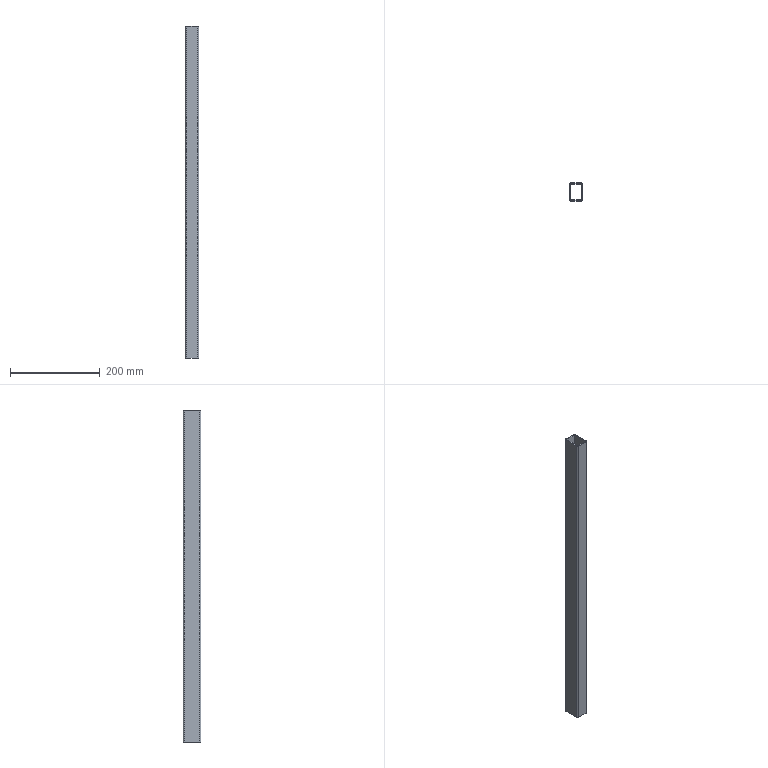Part | SolidWorks | features BaseBody 1 | 1 solid | 18 faces | box 30 x 40 x 740 mm | volume 234942 mm3 | plane 10 | cylinder 8 | commonest cylinder face diameters 1 x4 6 x4
STEP:
#1=CARTESIAN_POINT('',(12.,17.5,-370.));
#2=VERTEX_POINT('',#1);
#3=CARTESIAN_POINT('',(-12.,17.5,-370.));
#4=VERTEX_POINT('',#3);
#5=CARTESIAN_POINT('',(-12.,17.5,-370.));
#6=DIRECTION('',(-1.,0.,0.));
#7=VECTOR('',#6,1000.);
#8=LINE('',#5,#7);
#9=EDGE_CURVE('',#2,#4,#8,.T.);
#10=ORIENTED_EDGE('',*,*,#9,.F.);
#11=CARTESIAN_POINT('',(12.,17.5,370.));
#12=VERTEX_POINT('',#11);
#13=CARTESIAN_POINT('',(12.,17.5,370.));
#14=DIRECTION('',(0.,0.,-1.));
#15=VECTOR('',#14,1000.);
#16=LINE('',#13,#15);
#17=EDGE_CURVE('',#12,#2,#16,.T.);
#18=ORIENTED_EDGE('',*,*,#17,.F.);
#19=CARTESIAN_POINT('',(-12.,17.5,370.));
#20=VERTEX_POINT('',#19);
#21=CARTESIAN_POINT('',(-12.,17.5,370.));
#22=DIRECTION('',(-1.,0.,0.));
#23=VECTOR('',#22,1000.);
#24=LINE('',#21,#23);
#25=EDGE_CURVE('',#12,#20,#24,.T.);
#26=ORIENTED_EDGE('',*,*,#25,.T.);
#27=CARTESIAN_POINT('',(-12.,17.5,370.));
#28=DIRECTION('',(0.,0.,-1.));
#29=VECTOR('',#28,1000.);
#30=LINE('',#27,#29);
#31=EDGE_CURVE('',#20,#4,#30,.T.);
#32=ORIENTED_EDGE('',*,*,#31,.T.);
#33=EDGE_LOOP('',(#10,#18,#26,#32));
#34=FACE_OUTER_BOUND('',#33,.T.);
#35=CARTESIAN_POINT('',(-12.,17.5,370.));
#36=DIRECTION('',(0.,-1.,0.));
#37=DIRECTION('',(0.,0.,-1.));
#38=AXIS2_PLACEMENT_3D('',#35,#36,#37);
#39=PLANE('',#38);
#40=ADVANCED_FACE('',(#34),#39,.T.);
#41=CARTESIAN_POINT('',(12.5,17.,-370.));
#42=VERTEX_POINT('',#41);
#43=CARTESIAN_POINT('',(12.,17.,-370.));
#44=DIRECTION('',(0.,0.,1.));
#45=DIRECTION('',(-1.,0.,0.));
#46=AXIS2_PLACEMENT_3D('',#43,#44,#45);
#47=CIRCLE('',#46,0.5);
#48=EDGE_CURVE('',#42,#2,#47,.T.);
#49=ORIENTED_EDGE('',*,*,#48,.F.);
#50=CARTESIAN_POINT('',(12.5,17.,370.));
#51=VERTEX_POINT('',#50);
#52=CARTESIAN_POINT('',(12.5,17.,370.));
#53=DIRECTION('',(0.,0.,-1.));
#54=VECTOR('',#53,1000.);
#55=LINE('',#52,#54);
#56=EDGE_CURVE('',#51,#42,#55,.T.);
#57=ORIENTED_EDGE('',*,*,#56,.F.);
#58=CARTESIAN_POINT('',(12.,17.,370.));
#59=DIRECTION('',(0.,0.,1.));
#60=DIRECTION('',(-1.,0.,0.));
#61=AXIS2_PLACEMENT_3D('',#58,#59,#60);
#62=CIRCLE('',#61,0.5);
#63=EDGE_CURVE('',#51,#12,#62,.T.);
#64=ORIENTED_EDGE('',*,*,#63,.T.);
#65=ORIENTED_EDGE('',*,*,#17,.T.);
#66=EDGE_LOOP('',(#49,#57,#64,#65));
#67=FACE_OUTER_BOUND('',#66,.T.);
#68=CARTESIAN_POINT('',(12.,17.,370.));
#69=DIRECTION('',(0.,0.,-1.));
#70=DIRECTION('',(-1.,0.,0.));
#71=AXIS2_PLACEMENT_3D('',#68,#69,#70);
#72=CYLINDRICAL_SURFACE('',#71,0.5);
#73=ADVANCED_FACE('',(#67),#72,.F.);
#74=CARTESIAN_POINT('',(12.5,-17.,-370.));
#75=VERTEX_POINT('',#74);
#76=CARTESIAN_POINT('',(12.5,17.,-370.));
#77=DIRECTION('',(0.,1.,0.));
#78=VECTOR('',#77,1000.);
#79=LINE('',#76,#78);
#80=EDGE_CURVE('',#75,#42,#79,.T.);
#81=ORIENTED_EDGE('',*,*,#80,.F.);
#82=CARTESIAN_POINT('',(12.5,-17.,370.));
#83=VERTEX_POINT('',#82);
#84=CARTESIAN_POINT('',(12.5,-17.,370.));
#85=DIRECTION('',(0.,0.,-1.));
#86=VECTOR('',#85,1000.);
#87=LINE('',#84,#86);
#88=EDGE_CURVE('',#83,#75,#87,.T.);
#89=ORIENTED_EDGE('',*,*,#88,.F.);
#90=CARTESIAN_POINT('',(12.5,17.,370.));
#91=DIRECTION('',(0.,1.,0.));
#92=VECTOR('',#91,1000.);
#93=LINE('',#90,#92);
#94=EDGE_CURVE('',#83,#51,#93,.T.);
#95=ORIENTED_EDGE('',*,*,#94,.T.);
#96=ORIENTED_EDGE('',*,*,#56,.T.);
#97=EDGE_LOOP('',(#81,#89,#95,#96));
#98=FACE_OUTER_BOUND('',#97,.T.);
#99=CARTESIAN_POINT('',(12.5,17.,370.));
#100=DIRECTION('',(-1.,0.,0.));
#101=DIRECTION('',(0.,1.,0.));
#102=AXIS2_PLACEMENT_3D('',#99,#100,#101);
#103=PLANE('',#102);
#104=ADVANCED_FACE('',(#98),#103,.T.);
#105=CARTESIAN_POINT('',(12.,-17.5,-370.));
#106=VERTEX_POINT('',#105);
#107=CARTESIAN_POINT('',(12.,-17.,-370.));
#108=DIRECTION('',(0.,0.,1.));
#109=DIRECTION('',(1.,0.,0.));
#110=AXIS2_PLACEMENT_3D('',#107,#108,#109);
#111=CIRCLE('',#110,0.5);
#112=EDGE_CURVE('',#106,#75,#111,.T.);
#113=ORIENTED_EDGE('',*,*,#112,.F.);
#114=CARTESIAN_POINT('',(12.,-17.5,370.));
#115=VERTEX_POINT('',#114);
#116=CARTESIAN_POINT('',(12.,-17.5,370.));
#117=DIRECTION('',(0.,0.,-1.));
#118=VECTOR('',#117,1000.);
#119=LINE('',#116,#118);
#120=EDGE_CURVE('',#115,#106,#119,.T.);
#121=ORIENTED_EDGE('',*,*,#120,.F.);
#122=CARTESIAN_POINT('',(12.,-17.,370.));
#123=DIRECTION('',(0.,0.,1.));
#124=DIRECTION('',(1.,0.,0.));
#125=AXIS2_PLACEMENT_3D('',#122,#123,#124);
#126=CIRCLE('',#125,0.5);
#127=EDGE_CURVE('',#115,#83,#126,.T.);
#128=ORIENTED_EDGE('',*,*,#127,.T.);
#129=ORIENTED_EDGE('',*,*,#88,.T.);
#130=EDGE_LOOP('',(#113,#121,#128,#129));
#131=FACE_OUTER_BOUND('',#130,.T.);
#132=CARTESIAN_POINT('',(12.,-17.,370.));
#133=DIRECTION('',(0.,0.,-1.));
#134=DIRECTION('',(-1.,0.,0.));
#135=AXIS2_PLACEMENT_3D('',#132,#133,#134);
#136=CYLINDRICAL_SURFACE('',#135,0.5);
#137=ADVANCED_FACE('',(#131),#136,.F.);
#138=CARTESIAN_POINT('',(-12.,-17.5,-370.));
#139=VERTEX_POINT('',#138);
#140=CARTESIAN_POINT('',(-12.,-17.5,-370.));
#141=DIRECTION('',(1.,0.,0.));
#142=VECTOR('',#141,1000.);
#143=LINE('',#140,#142);
#144=EDGE_CURVE('',#139,#106,#143,.T.);
#145=ORIENTED_EDGE('',*,*,#144,.F.);
#146=CARTESIAN_POINT('',(-12.,-17.5,370.));
#147=VERTEX_POINT('',#146);
#148=CARTESIAN_POINT('',(-12.,-17.5,370.));
#149=DIRECTION('',(0.,0.,-1.));
#150=VECTOR('',#149,1000.);
#151=LINE('',#148,#150);
#152=EDGE_CURVE('',#147,#139,#151,.T.);
#153=ORIENTED_EDGE('',*,*,#152,.F.);
#154=CARTESIAN_POINT('',(-12.,-17.5,370.));
#155=DIRECTION('',(1.,0.,0.));
#156=VECTOR('',#155,1000.);
#157=LINE('',#154,#156);
#158=EDGE_CURVE('',#147,#115,#157,.T.);
#159=ORIENTED_EDGE('',*,*,#158,.T.);
#160=ORIENTED_EDGE('',*,*,#120,.T.);
#161=EDGE_LOOP('',(#145,#153,#159,#160));
#162=FACE_OUTER_BOUND('',#161,.T.);
#163=CARTESIAN_POINT('',(-12.,-17.5,370.));
#164=DIRECTION('',(0.,1.,0.));
#165=DIRECTION('',(1.,0.,0.));
#166=AXIS2_PLACEMENT_3D('',#163,#164,#165);
#167=PLANE('',#166);
#168=ADVANCED_FACE('',(#162),#167,.T.);
#169=CARTESIAN_POINT('',(-12.5,-17.,-370.));
#170=VERTEX_POINT('',#169);
#171=CARTESIAN_POINT('',(-12.,-17.,-370.));
#172=DIRECTION('',(0.,0.,1.));
#173=DIRECTION('',(1.,0.,0.));
#174=AXIS2_PLACEMENT_3D('',#171,#172,#173);
#175=CIRCLE('',#174,0.5);
#176=EDGE_CURVE('',#170,#139,#175,.T.);
#177=ORIENTED_EDGE('',*,*,#176,.F.);
#178=CARTESIAN_POINT('',(-12.5,-17.,370.));
#179=VERTEX_POINT('',#178);
#180=CARTESIAN_POINT('',(-12.5,-17.,370.));
#181=DIRECTION('',(0.,0.,-1.));
#182=VECTOR('',#181,1000.);
#183=LINE('',#180,#182);
#184=EDGE_CURVE('',#179,#170,#183,.T.);
#185=ORIENTED_EDGE('',*,*,#184,.F.);
#186=CARTESIAN_POINT('',(-12.,-17.,370.));
#187=DIRECTION('',(0.,0.,1.));
#188=DIRECTION('',(1.,0.,0.));
#189=AXIS2_PLACEMENT_3D('',#186,#187,#188);
#190=CIRCLE('',#189,0.5);
#191=EDGE_CURVE('',#179,#147,#190,.T.);
#192=ORIENTED_EDGE('',*,*,#191,.T.);
#193=ORIENTED_EDGE('',*,*,#152,.T.);
#194=EDGE_LOOP('',(#177,#185,#192,#193));
#195=FACE_OUTER_BOUND('',#194,.T.);
#196=CARTESIAN_POINT('',(-12.,-17.,370.));
#197=DIRECTION('',(0.,0.,-1.));
#198=DIRECTION('',(-1.,0.,0.));
#199=AXIS2_PLACEMENT_3D('',#196,#197,#198);
#200=CYLINDRICAL_SURFACE('',#199,0.5);
#201=ADVANCED_FACE('',(#195),#200,.F.);
#202=CARTESIAN_POINT('',(-12.5,17.,-370.));
#203=VERTEX_POINT('',#202);
#204=CARTESIAN_POINT('',(-12.5,17.,-370.));
#205=DIRECTION('',(0.,-1.,0.));
#206=VECTOR('',#205,1000.);
#207=LINE('',#204,#206);
#208=EDGE_CURVE('',#203,#170,#207,.T.);
#209=ORIENTED_EDGE('',*,*,#208,.F.);
#210=CARTESIAN_POINT('',(-12.5,17.,370.));
#211=VERTEX_POINT('',#210);
#212=CARTESIAN_POINT('',(-12.5,17.,370.));
#213=DIRECTION('',(0.,0.,-1.));
#214=VECTOR('',#213,1000.);
#215=LINE('',#212,#214);
#216=EDGE_CURVE('',#211,#203,#215,.T.);
#217=ORIENTED_EDGE('',*,*,#216,.F.);
#218=CARTESIAN_POINT('',(-12.5,17.,370.));
#219=DIRECTION('',(0.,-1.,0.));
#220=VECTOR('',#219,1000.);
#221=LINE('',#218,#220);
#222=EDGE_CURVE('',#211,#179,#221,.T.);
#223=ORIENTED_EDGE('',*,*,#222,.T.);
#224=ORIENTED_EDGE('',*,*,#184,.T.);
#225=EDGE_LOOP('',(#209,#217,#223,#224));
#226=FACE_OUTER_BOUND('',#225,.T.);
#227=CARTESIAN_POINT('',(-12.5,17.,370.));
#228=DIRECTION('',(1.,0.,0.));
#229=DIRECTION('',(0.,1.,0.));
#230=AXIS2_PLACEMENT_3D('',#227,#228,#229);
#231=PLANE('',#230);
#232=ADVANCED_FACE('',(#226),#231,.T.);
#233=CARTESIAN_POINT('',(-12.,17.,-370.));
#234=DIRECTION('',(0.,0.,1.));
#235=DIRECTION('',(1.,0.,0.));
#236=AXIS2_PLACEMENT_3D('',#233,#234,#235);
#237=CIRCLE('',#236,0.5);
#238=EDGE_CURVE('',#4,#203,#237,.T.);
#239=ORIENTED_EDGE('',*,*,#238,.F.);
#240=ORIENTED_EDGE('',*,*,#31,.F.);
#241=CARTESIAN_POINT('',(-12.,17.,370.));
#242=DIRECTION('',(0.,0.,1.));
#243=DIRECTION('',(1.,0.,0.));
#244=AXIS2_PLACEMENT_3D('',#241,#242,#243);
#245=CIRCLE('',#244,0.5);
#246=EDGE_CURVE('',#20,#211,#245,.T.);
#247=ORIENTED_EDGE('',*,*,#246,.T.);
#248=ORIENTED_EDGE('',*,*,#216,.T.);
#249=EDGE_LOOP('',(#239,#240,#247,#248));
#250=FACE_OUTER_BOUND('',#249,.T.);
#251=CARTESIAN_POINT('',(-12.,17.,370.));
#252=DIRECTION('',(0.,0.,-1.));
#253=DIRECTION('',(-1.,0.,0.));
#254=AXIS2_PLACEMENT_3D('',#251,#252,#253);
#255=CYLINDRICAL_SURFACE('',#254,0.5);
#256=ADVANCED_FACE('',(#250),#255,.F.);
#257=CARTESIAN_POINT('',(-15.,17.,-370.));
#258=VERTEX_POINT('',#257);
#259=CARTESIAN_POINT('',(-15.,-17.,-370.));
#260=VERTEX_POINT('',#259);
#261=CARTESIAN_POINT('',(-15.,17.,-370.));
#262=DIRECTION('',(0.,-1.,0.));
#263=VECTOR('',#262,1000.);
#264=LINE('',#261,#263);
#265=EDGE_CURVE('',#258,#260,#264,.T.);
#266=ORIENTED_EDGE('',*,*,#265,.T.);
#267=CARTESIAN_POINT('',(-15.,-17.,370.));
#268=VERTEX_POINT('',#267);
#269=CARTESIAN_POINT('',(-15.,-17.,370.));
#270=DIRECTION('',(0.,0.,-1.));
#271=VECTOR('',#270,1000.);
#272=LINE('',#269,#271);
#273=EDGE_CURVE('',#268,#260,#272,.T.);
#274=ORIENTED_EDGE('',*,*,#273,.F.);
#275=CARTESIAN_POINT('',(-15.,17.,370.));
#276=VERTEX_POINT('',#275);
#277=CARTESIAN_POINT('',(-15.,17.,370.));
#278=DIRECTION('',(0.,-1.,0.));
#279=VECTOR('',#278,1000.);
#280=LINE('',#277,#279);
#281=EDGE_CURVE('',#276,#268,#280,.T.);
#282=ORIENTED_EDGE('',*,*,#281,.F.);
#283=CARTESIAN_POINT('',(-15.,17.,370.));
#284=DIRECTION('',(0.,0.,-1.));
#285=VECTOR('',#284,1000.);
#286=LINE('',#283,#285);
#287=EDGE_CURVE('',#276,#258,#286,.T.);
#288=ORIENTED_EDGE('',*,*,#287,.T.);
#289=EDGE_LOOP('',(#266,#274,#282,#288));
#290=FACE_OUTER_BOUND('',#289,.T.);
#291=CARTESIAN_POINT('',(-15.,17.,370.));
#292=DIRECTION('',(1.,0.,0.));
#293=DIRECTION('',(0.,1.,0.));
#294=AXIS2_PLACEMENT_3D('',#291,#292,#293);
#295=PLANE('',#294);
#296=ADVANCED_FACE('',(#290),#295,.F.);
#297=CARTESIAN_POINT('',(-12.,20.,-370.));
#298=VERTEX_POINT('',#297);
#299=CARTESIAN_POINT('',(-12.,17.,-370.));
#300=DIRECTION('',(0.,0.,1.));
#301=DIRECTION('',(1.,0.,0.));
#302=AXIS2_PLACEMENT_3D('',#299,#300,#301);
#303=CIRCLE('',#302,3.);
#304=EDGE_CURVE('',#298,#258,#303,.T.);
#305=ORIENTED_EDGE('',*,*,#304,.T.);
#306=ORIENTED_EDGE('',*,*,#287,.F.);
#307=CARTESIAN_POINT('',(-12.,20.,370.));
#308=VERTEX_POINT('',#307);
#309=CARTESIAN_POINT('',(-12.,17.,370.));
#310=DIRECTION('',(0.,0.,1.));
#311=DIRECTION('',(1.,0.,0.));
#312=AXIS2_PLACEMENT_3D('',#309,#310,#311);
#313=CIRCLE('',#312,3.);
#314=EDGE_CURVE('',#308,#276,#313,.T.);
#315=ORIENTED_EDGE('',*,*,#314,.F.);
#316=CARTESIAN_POINT('',(-12.,20.,370.));
#317=DIRECTION('',(0.,0.,-1.));
#318=VECTOR('',#317,1000.);
#319=LINE('',#316,#318);
#320=EDGE_CURVE('',#308,#298,#319,.T.);
#321=ORIENTED_EDGE('',*,*,#320,.T.);
#322=EDGE_LOOP('',(#305,#306,#315,#321));
#323=FACE_OUTER_BOUND('',#322,.T.);
#324=CARTESIAN_POINT('',(-12.,17.,370.));
#325=DIRECTION('',(0.,0.,-1.));
#326=DIRECTION('',(-1.,0.,0.));
#327=AXIS2_PLACEMENT_3D('',#324,#325,#326);
#328=CYLINDRICAL_SURFACE('',#327,3.);
#329=ADVANCED_FACE('',(#323),#328,.T.);
#330=CARTESIAN_POINT('',(12.,20.,-370.));
#331=VERTEX_POINT('',#330);
#332=CARTESIAN_POINT('',(-12.,20.,-370.));
#333=DIRECTION('',(-1.,0.,0.));
#334=VECTOR('',#333,1000.);
#335=LINE('',#332,#334);
#336=EDGE_CURVE('',#331,#298,#335,.T.);
#337=ORIENTED_EDGE('',*,*,#336,.T.);
#338=ORIENTED_EDGE('',*,*,#320,.F.);
#339=CARTESIAN_POINT('',(12.,20.,370.));
#340=VERTEX_POINT('',#339);
#341=CARTESIAN_POINT('',(-12.,20.,370.));
#342=DIRECTION('',(-1.,0.,0.));
#343=VECTOR('',#342,1000.);
#344=LINE('',#341,#343);
#345=EDGE_CURVE('',#340,#308,#344,.T.);
#346=ORIENTED_EDGE('',*,*,#345,.F.);
#347=CARTESIAN_POINT('',(12.,20.,370.));
#348=DIRECTION('',(0.,0.,-1.));
#349=VECTOR('',#348,1000.);
#350=LINE('',#347,#349);
#351=EDGE_CURVE('',#340,#331,#350,.T.);
#352=ORIENTED_EDGE('',*,*,#351,.T.);
#353=EDGE_LOOP('',(#337,#338,#346,#352));
#354=FACE_OUTER_BOUND('',#353,.T.);
#355=CARTESIAN_POINT('',(-12.,20.,370.));
#356=DIRECTION('',(0.,-1.,0.));
#357=DIRECTION('',(0.,0.,-1.));
#358=AXIS2_PLACEMENT_3D('',#355,#356,#357);
#359=PLANE('',#358);
#360=ADVANCED_FACE('',(#354),#359,.F.);
#361=CARTESIAN_POINT('',(15.,17.,-370.));
#362=VERTEX_POINT('',#361);
#363=CARTESIAN_POINT('',(12.,17.,-370.));
#364=DIRECTION('',(0.,0.,1.));
#365=DIRECTION('',(-1.,0.,0.));
#366=AXIS2_PLACEMENT_3D('',#363,#364,#365);
#367=CIRCLE('',#366,3.);
#368=EDGE_CURVE('',#362,#331,#367,.T.);
#369=ORIENTED_EDGE('',*,*,#368,.T.);
#370=ORIENTED_EDGE('',*,*,#351,.F.);
#371=CARTESIAN_POINT('',(15.,17.,370.));
#372=VERTEX_POINT('',#371);
#373=CARTESIAN_POINT('',(12.,17.,370.));
#374=DIRECTION('',(0.,0.,1.));
#375=DIRECTION('',(-1.,0.,0.));
#376=AXIS2_PLACEMENT_3D('',#373,#374,#375);
#377=CIRCLE('',#376,3.);
#378=EDGE_CURVE('',#372,#340,#377,.T.);
#379=ORIENTED_EDGE('',*,*,#378,.F.);
#380=CARTESIAN_POINT('',(15.,17.,370.));
#381=DIRECTION('',(0.,0.,-1.));
#382=VECTOR('',#381,1000.);
#383=LINE('',#380,#382);
#384=EDGE_CURVE('',#372,#362,#383,.T.);
#385=ORIENTED_EDGE('',*,*,#384,.T.);
#386=EDGE_LOOP('',(#369,#370,#379,#385));
#387=FACE_OUTER_BOUND('',#386,.T.);
#388=CARTESIAN_POINT('',(12.,17.,370.));
#389=DIRECTION('',(0.,0.,-1.));
#390=DIRECTION('',(-1.,0.,0.));
#391=AXIS2_PLACEMENT_3D('',#388,#389,#390);
#392=CYLINDRICAL_SURFACE('',#391,3.);
#393=ADVANCED_FACE('',(#387),#392,.T.);
#394=CARTESIAN_POINT('',(15.,-17.,-370.));
#395=VERTEX_POINT('',#394);
#396=CARTESIAN_POINT('',(15.,17.,-370.));
#397=DIRECTION('',(0.,1.,0.));
#398=VECTOR('',#397,1000.);
#399=LINE('',#396,#398);
#400=EDGE_CURVE('',#395,#362,#399,.T.);
#401=ORIENTED_EDGE('',*,*,#400,.T.);
#402=ORIENTED_EDGE('',*,*,#384,.F.);
#403=CARTESIAN_POINT('',(15.,-17.,370.));
#404=VERTEX_POINT('',#403);
#405=CARTESIAN_POINT('',(15.,17.,370.));
#406=DIRECTION('',(0.,1.,0.));
#407=VECTOR('',#406,1000.);
#408=LINE('',#405,#407);
#409=EDGE_CURVE('',#404,#372,#408,.T.);
#410=ORIENTED_EDGE('',*,*,#409,.F.);
#411=CARTESIAN_POINT('',(15.,-17.,370.));
#412=DIRECTION('',(0.,0.,-1.));
#413=VECTOR('',#412,1000.);
#414=LINE('',#411,#413);
#415=EDGE_CURVE('',#404,#395,#414,.T.);
#416=ORIENTED_EDGE('',*,*,#415,.T.);
#417=EDGE_LOOP('',(#401,#402,#410,#416));
#418=FACE_OUTER_BOUND('',#417,.T.);
#419=CARTESIAN_POINT('',(15.,17.,370.));
#420=DIRECTION('',(-1.,0.,0.));
#421=DIRECTION('',(0.,1.,0.));
#422=AXIS2_PLACEMENT_3D('',#419,#420,#421);
#423=PLANE('',#422);
#424=ADVANCED_FACE('',(#418),#423,.F.);
#425=CARTESIAN_POINT('',(12.,-20.,-370.));
#426=VERTEX_POINT('',#425);
#427=CARTESIAN_POINT('',(12.,-17.,-370.));
#428=DIRECTION('',(0.,0.,1.));
#429=DIRECTION('',(1.,0.,0.));
#430=AXIS2_PLACEMENT_3D('',#427,#428,#429);
#431=CIRCLE('',#430,3.);
#432=EDGE_CURVE('',#426,#395,#431,.T.);
#433=ORIENTED_EDGE('',*,*,#432,.T.);
#434=ORIENTED_EDGE('',*,*,#415,.F.);
#435=CARTESIAN_POINT('',(12.,-20.,370.));
#436=VERTEX_POINT('',#435);
#437=CARTESIAN_POINT('',(12.,-17.,370.));
#438=DIRECTION('',(0.,0.,1.));
#439=DIRECTION('',(1.,0.,0.));
#440=AXIS2_PLACEMENT_3D('',#437,#438,#439);
#441=CIRCLE('',#440,3.);
#442=EDGE_CURVE('',#436,#404,#441,.T.);
#443=ORIENTED_EDGE('',*,*,#442,.F.);
#444=CARTESIAN_POINT('',(12.,-20.,370.));
#445=DIRECTION('',(0.,0.,-1.));
#446=VECTOR('',#445,1000.);
#447=LINE('',#444,#446);
#448=EDGE_CURVE('',#436,#426,#447,.T.);
#449=ORIENTED_EDGE('',*,*,#448,.T.);
#450=EDGE_LOOP('',(#433,#434,#443,#449));
#451=FACE_OUTER_BOUND('',#450,.T.);
#452=CARTESIAN_POINT('',(12.,-17.,370.));
#453=DIRECTION('',(0.,0.,-1.));
#454=DIRECTION('',(-1.,0.,0.));
#455=AXIS2_PLACEMENT_3D('',#452,#453,#454);
#456=CYLINDRICAL_SURFACE('',#455,3.);
#457=ADVANCED_FACE('',(#451),#456,.T.);
#458=CARTESIAN_POINT('',(-12.,-20.,-370.));
#459=VERTEX_POINT('',#458);
#460=CARTESIAN_POINT('',(-12.,-20.,-370.));
#461=DIRECTION('',(1.,0.,0.));
#462=VECTOR('',#461,1000.);
#463=LINE('',#460,#462);
#464=EDGE_CURVE('',#459,#426,#463,.T.);
#465=ORIENTED_EDGE('',*,*,#464,.T.);
#466=ORIENTED_EDGE('',*,*,#448,.F.);
#467=CARTESIAN_POINT('',(-12.,-20.,370.));
#468=VERTEX_POINT('',#467);
#469=CARTESIAN_POINT('',(-12.,-20.,370.));
#470=DIRECTION('',(1.,0.,0.));
#471=VECTOR('',#470,1000.);
#472=LINE('',#469,#471);
#473=EDGE_CURVE('',#468,#436,#472,.T.);
#474=ORIENTED_EDGE('',*,*,#473,.F.);
#475=CARTESIAN_POINT('',(-12.,-20.,370.));
#476=DIRECTION('',(0.,0.,-1.));
#477=VECTOR('',#476,1000.);
#478=LINE('',#475,#477);
#479=EDGE_CURVE('',#468,#459,#478,.T.);
#480=ORIENTED_EDGE('',*,*,#479,.T.);
#481=EDGE_LOOP('',(#465,#466,#474,#480));
#482=FACE_OUTER_BOUND('',#481,.T.);
#483=CARTESIAN_POINT('',(-12.,-20.,370.));
#484=DIRECTION('',(0.,1.,0.));
#485=DIRECTION('',(1.,0.,0.));
#486=AXIS2_PLACEMENT_3D('',#483,#484,#485);
#487=PLANE('',#486);
#488=ADVANCED_FACE('',(#482),#487,.F.);
#489=CARTESIAN_POINT('',(-12.,-17.,-370.));
#490=DIRECTION('',(0.,0.,1.));
#491=DIRECTION('',(1.,0.,0.));
#492=AXIS2_PLACEMENT_3D('',#489,#490,#491);
#493=CIRCLE('',#492,3.);
#494=EDGE_CURVE('',#260,#459,#493,.T.);
#495=ORIENTED_EDGE('',*,*,#494,.T.);
#496=ORIENTED_EDGE('',*,*,#479,.F.);
#497=CARTESIAN_POINT('',(-12.,-17.,370.));
#498=DIRECTION('',(0.,0.,1.));
#499=DIRECTION('',(1.,0.,0.));
#500=AXIS2_PLACEMENT_3D('',#497,#498,#499);
#501=CIRCLE('',#500,3.);
#502=EDGE_CURVE('',#268,#468,#501,.T.);
#503=ORIENTED_EDGE('',*,*,#502,.F.);
#504=ORIENTED_EDGE('',*,*,#273,.T.);
#505=EDGE_LOOP('',(#495,#496,#503,#504));
#506=FACE_OUTER_BOUND('',#505,.T.);
#507=CARTESIAN_POINT('',(-12.,-17.,370.));
#508=DIRECTION('',(0.,0.,-1.));
#509=DIRECTION('',(-1.,0.,0.));
#510=AXIS2_PLACEMENT_3D('',#507,#508,#509);
#511=CYLINDRICAL_SURFACE('',#510,3.);
#512=ADVANCED_FACE('',(#506),#511,.T.);
#513=ORIENTED_EDGE('',*,*,#238,.T.);
#514=ORIENTED_EDGE('',*,*,#208,.T.);
#515=ORIENTED_EDGE('',*,*,#176,.T.);
#516=ORIENTED_EDGE('',*,*,#144,.T.);
#517=ORIENTED_EDGE('',*,*,#112,.T.);
#518=ORIENTED_EDGE('',*,*,#80,.T.);
#519=ORIENTED_EDGE('',*,*,#48,.T.);
#520=ORIENTED_EDGE('',*,*,#9,.T.);
#521=EDGE_LOOP('',(#513,#514,#515,#516,#517,#518,#519,#520));
#522=FACE_BOUND('',#521,.T.);
#523=ORIENTED_EDGE('',*,*,#494,.F.);
#524=ORIENTED_EDGE('',*,*,#265,.F.);
#525=ORIENTED_EDGE('',*,*,#304,.F.);
#526=ORIENTED_EDGE('',*,*,#336,.F.);
#527=ORIENTED_EDGE('',*,*,#368,.F.);
#528=ORIENTED_EDGE('',*,*,#400,.F.);
#529=ORIENTED_EDGE('',*,*,#432,.F.);
#530=ORIENTED_EDGE('',*,*,#464,.F.);
#531=EDGE_LOOP('',(#523,#524,#525,#526,#527,#528,#529,#530));
#532=FACE_OUTER_BOUND('',#531,.T.);
#533=CARTESIAN_POINT('',(-12.,-17.,-370.));
#534=DIRECTION('',(0.,0.,1.));
#535=DIRECTION('',(1.,0.,0.));
#536=AXIS2_PLACEMENT_3D('',#533,#534,#535);
#537=PLANE('',#536);
#538=ADVANCED_FACE('',(#522,#532),#537,.F.);
#539=ORIENTED_EDGE('',*,*,#222,.F.);
#540=ORIENTED_EDGE('',*,*,#246,.F.);
#541=ORIENTED_EDGE('',*,*,#25,.F.);
#542=ORIENTED_EDGE('',*,*,#63,.F.);
#543=ORIENTED_EDGE('',*,*,#94,.F.);
#544=ORIENTED_EDGE('',*,*,#127,.F.);
#545=ORIENTED_EDGE('',*,*,#158,.F.);
#546=ORIENTED_EDGE('',*,*,#191,.F.);
#547=EDGE_LOOP('',(#539,#540,#541,#542,#543,#544,#545,#546));
#548=FACE_BOUND('',#547,.T.);
#549=ORIENTED_EDGE('',*,*,#502,.T.);
#550=ORIENTED_EDGE('',*,*,#473,.T.);
#551=ORIENTED_EDGE('',*,*,#442,.T.);
#552=ORIENTED_EDGE('',*,*,#409,.T.);
#553=ORIENTED_EDGE('',*,*,#378,.T.);
#554=ORIENTED_EDGE('',*,*,#345,.T.);
#555=ORIENTED_EDGE('',*,*,#314,.T.);
#556=ORIENTED_EDGE('',*,*,#281,.T.);
#557=EDGE_LOOP('',(#549,#550,#551,#552,#553,#554,#555,#556));
#558=FACE_OUTER_BOUND('',#557,.T.);
#559=CARTESIAN_POINT('',(-12.,-17.,370.));
#560=DIRECTION('',(0.,0.,1.));
#561=DIRECTION('',(1.,0.,0.));
#562=AXIS2_PLACEMENT_3D('',#559,#560,#561);
#563=PLANE('',#562);
#564=ADVANCED_FACE('',(#548,#558),#563,.T.);
#565=CLOSED_SHELL('',(#40,#73,#104,#137,#168,#201,#232,#256,#296,#329,#360,#393,#424,#457,#488,#512,#538,#564));
#566=MANIFOLD_SOLID_BREP('',#565);
#567=CARTESIAN_POINT('',(0.,0.,0.));
#568=DIRECTION('',(0.,0.,1.));
#569=DIRECTION('',(1.,0.,0.));
#570=AXIS2_PLACEMENT_3D('',#567,#568,#569);
#571=(LENGTH_UNIT()NAMED_UNIT(*)SI_UNIT(.MILLI.,.METRE.));
#572=UNCERTAINTY_MEASURE_WITH_UNIT(LENGTH_MEASURE(0.00001),#571,'','');
#573=(NAMED_UNIT(*)PLANE_ANGLE_UNIT()SI_UNIT($,.RADIAN.));
#574=(NAMED_UNIT(*)SI_UNIT($,.STERADIAN.)SOLID_ANGLE_UNIT());
#575=(GEOMETRIC_REPRESENTATION_CONTEXT(3)GLOBAL_UNCERTAINTY_ASSIGNED_CONTEXT((#572))GLOBAL_UNIT_ASSIGNED_CONTEXT((#571,#573,#574))REPRESENTATION_CONTEXT('',''));
#576=ADVANCED_BREP_SHAPE_REPRESENTATION('',(#566,#570),#575);